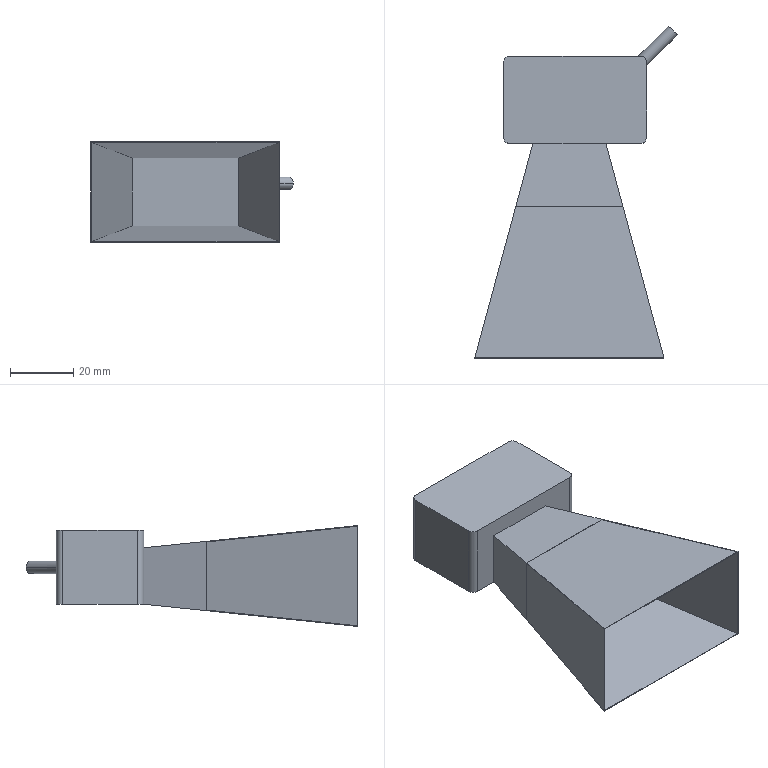Part | SolidWorks | features Blend 2, Extrusion 1, HoleWzd 1, ICE 1, Shell 1, Sweep 1 | 3 solids | 41 faces | box 64.206 x 105.323 x 32 mm | volume 42247 mm3 | plane 24 | cylinder 13 | cone 4 | commonest cylinder face diameters 4 x7 2.5 x4 7.5 x2
STEP:
#1=CARTESIAN_POINT('',(17.125,9.35,-3.25));
#2=VERTEX_POINT('',#1);
#3=CARTESIAN_POINT('',(14.625,9.35,-3.25));
#4=VERTEX_POINT('',#3);
#5=CARTESIAN_POINT('',(15.875,9.35,-3.25));
#6=DIRECTION('',(0.,0.,-1.));
#7=DIRECTION('',(-1.,0.,0.));
#8=AXIS2_PLACEMENT_3D('',#5,#6,#7);
#9=CIRCLE('',#8,1.25);
#10=EDGE_CURVE('',#2,#4,#9,.T.);
#11=ORIENTED_EDGE('',*,*,#10,.F.);
#12=CARTESIAN_POINT('',(17.125,9.35,-11.75));
#13=VERTEX_POINT('',#12);
#14=CARTESIAN_POINT('',(17.125,9.35,-11.75));
#15=DIRECTION('',(0.,0.,-1.));
#16=VECTOR('',#15,1000.);
#17=LINE('',#14,#16);
#18=EDGE_CURVE('',#2,#13,#17,.T.);
#19=ORIENTED_EDGE('',*,*,#18,.T.);
#20=CARTESIAN_POINT('',(14.625,9.35,-11.75));
#21=VERTEX_POINT('',#20);
#22=CARTESIAN_POINT('',(15.875,9.35,-11.75));
#23=DIRECTION('',(0.,0.,-1.));
#24=DIRECTION('',(-1.,0.,0.));
#25=AXIS2_PLACEMENT_3D('',#22,#23,#24);
#26=CIRCLE('',#25,1.25);
#27=EDGE_CURVE('',#13,#21,#26,.T.);
#28=ORIENTED_EDGE('',*,*,#27,.T.);
#29=CARTESIAN_POINT('',(14.625,9.35,-11.75));
#30=DIRECTION('',(0.,0.,-1.));
#31=VECTOR('',#30,1000.);
#32=LINE('',#29,#31);
#33=EDGE_CURVE('',#4,#21,#32,.T.);
#34=ORIENTED_EDGE('',*,*,#33,.F.);
#35=EDGE_LOOP('',(#11,#19,#28,#34));
#36=FACE_OUTER_BOUND('',#35,.T.);
#37=CARTESIAN_POINT('',(15.875,9.35,-11.75));
#38=DIRECTION('',(0.,0.,-1.));
#39=DIRECTION('',(-1.,0.,0.));
#40=AXIS2_PLACEMENT_3D('',#37,#38,#39);
#41=CYLINDRICAL_SURFACE('',#40,1.25);
#42=ADVANCED_FACE('',(#36),#41,.F.);
#43=CARTESIAN_POINT('',(15.875,9.35,-2.499));
#44=VERTEX_POINT('',#43);
#45=CARTESIAN_POINT('',(14.625,9.35,-3.25));
#46=DIRECTION('',(-0.8572,0.,-0.515));
#47=VECTOR('',#46,1000.);
#48=LINE('',#45,#47);
#49=EDGE_CURVE('',#44,#4,#48,.T.);
#50=ORIENTED_EDGE('',*,*,#49,.F.);
#51=CARTESIAN_POINT('',(17.125,9.35,-3.25));
#52=DIRECTION('',(0.8572,0.,-0.515));
#53=VECTOR('',#52,1000.);
#54=LINE('',#51,#53);
#55=EDGE_CURVE('',#44,#2,#54,.T.);
#56=ORIENTED_EDGE('',*,*,#55,.T.);
#57=ORIENTED_EDGE('',*,*,#10,.T.);
#58=EDGE_LOOP('',(#50,#56,#57));
#59=FACE_OUTER_BOUND('',#58,.T.);
#60=CARTESIAN_POINT('',(15.875,9.35,-3.25));
#61=DIRECTION('',(0.,0.,-1.));
#62=DIRECTION('',(-1.,0.,0.));
#63=AXIS2_PLACEMENT_3D('',#60,#61,#62);
#64=CONICAL_SURFACE('',#63,1.25,1.03);
#65=ADVANCED_FACE('',(#59),#64,.F.);
#66=CARTESIAN_POINT('',(-14.625,9.35,-3.25));
#67=VERTEX_POINT('',#66);
#68=CARTESIAN_POINT('',(-17.125,9.35,-3.25));
#69=VERTEX_POINT('',#68);
#70=CARTESIAN_POINT('',(-15.875,9.35,-3.25));
#71=DIRECTION('',(0.,0.,-1.));
#72=DIRECTION('',(-1.,0.,0.));
#73=AXIS2_PLACEMENT_3D('',#70,#71,#72);
#74=CIRCLE('',#73,1.25);
#75=EDGE_CURVE('',#67,#69,#74,.T.);
#76=ORIENTED_EDGE('',*,*,#75,.F.);
#77=CARTESIAN_POINT('',(-14.625,9.35,-11.75));
#78=VERTEX_POINT('',#77);
#79=CARTESIAN_POINT('',(-14.625,9.35,-11.75));
#80=DIRECTION('',(0.,0.,-1.));
#81=VECTOR('',#80,1000.);
#82=LINE('',#79,#81);
#83=EDGE_CURVE('',#67,#78,#82,.T.);
#84=ORIENTED_EDGE('',*,*,#83,.T.);
#85=CARTESIAN_POINT('',(-17.125,9.35,-11.75));
#86=VERTEX_POINT('',#85);
#87=CARTESIAN_POINT('',(-15.875,9.35,-11.75));
#88=DIRECTION('',(0.,0.,-1.));
#89=DIRECTION('',(-1.,0.,0.));
#90=AXIS2_PLACEMENT_3D('',#87,#88,#89);
#91=CIRCLE('',#90,1.25);
#92=EDGE_CURVE('',#78,#86,#91,.T.);
#93=ORIENTED_EDGE('',*,*,#92,.T.);
#94=CARTESIAN_POINT('',(-17.125,9.35,-11.75));
#95=DIRECTION('',(0.,0.,-1.));
#96=VECTOR('',#95,1000.);
#97=LINE('',#94,#96);
#98=EDGE_CURVE('',#69,#86,#97,.T.);
#99=ORIENTED_EDGE('',*,*,#98,.F.);
#100=EDGE_LOOP('',(#76,#84,#93,#99));
#101=FACE_OUTER_BOUND('',#100,.T.);
#102=CARTESIAN_POINT('',(-15.875,9.35,-11.75));
#103=DIRECTION('',(0.,0.,-1.));
#104=DIRECTION('',(-1.,0.,0.));
#105=AXIS2_PLACEMENT_3D('',#102,#103,#104);
#106=CYLINDRICAL_SURFACE('',#105,1.25);
#107=ADVANCED_FACE('',(#101),#106,.F.);
#108=CARTESIAN_POINT('',(-15.875,9.35,-2.499));
#109=VERTEX_POINT('',#108);
#110=CARTESIAN_POINT('',(-17.125,9.35,-3.25));
#111=DIRECTION('',(-0.8572,0.,-0.515));
#112=VECTOR('',#111,1000.);
#113=LINE('',#110,#112);
#114=EDGE_CURVE('',#109,#69,#113,.T.);
#115=ORIENTED_EDGE('',*,*,#114,.F.);
#116=CARTESIAN_POINT('',(-14.625,9.35,-3.25));
#117=DIRECTION('',(0.8572,0.,-0.515));
#118=VECTOR('',#117,1000.);
#119=LINE('',#116,#118);
#120=EDGE_CURVE('',#109,#67,#119,.T.);
#121=ORIENTED_EDGE('',*,*,#120,.T.);
#122=ORIENTED_EDGE('',*,*,#75,.T.);
#123=EDGE_LOOP('',(#115,#121,#122));
#124=FACE_OUTER_BOUND('',#123,.T.);
#125=CARTESIAN_POINT('',(-15.875,9.35,-3.25));
#126=DIRECTION('',(0.,0.,-1.));
#127=DIRECTION('',(-1.,0.,0.));
#128=AXIS2_PLACEMENT_3D('',#125,#126,#127);
#129=CONICAL_SURFACE('',#128,1.25,1.03);
#130=ADVANCED_FACE('',(#124),#129,.F.);
#131=CARTESIAN_POINT('',(-1.8,-8.85,1.));
#132=VERTEX_POINT('',#131);
#133=CARTESIAN_POINT('',(-1.8,-8.85,-6.5));
#134=VERTEX_POINT('',#133);
#135=CARTESIAN_POINT('',(-1.8,-8.85,-2.75));
#136=DIRECTION('',(0.,-1.,0.));
#137=DIRECTION('',(0.,0.,-1.));
#138=AXIS2_PLACEMENT_3D('',#135,#136,#137);
#139=CIRCLE('',#138,3.75);
#140=EDGE_CURVE('',#132,#134,#139,.T.);
#141=ORIENTED_EDGE('',*,*,#140,.F.);
#142=CARTESIAN_POINT('',(-1.8,-13.85,1.));
#143=VERTEX_POINT('',#142);
#144=CARTESIAN_POINT('',(-1.8,-8.85,1.));
#145=DIRECTION('',(0.,-1.,0.));
#146=VECTOR('',#145,1000.);
#147=LINE('',#144,#146);
#148=EDGE_CURVE('',#132,#143,#147,.T.);
#149=ORIENTED_EDGE('',*,*,#148,.T.);
#150=CARTESIAN_POINT('',(-1.8,-13.85,-6.5));
#151=VERTEX_POINT('',#150);
#152=CARTESIAN_POINT('',(-1.8,-13.85,-2.75));
#153=DIRECTION('',(0.,-1.,0.));
#154=DIRECTION('',(0.,0.,-1.));
#155=AXIS2_PLACEMENT_3D('',#152,#153,#154);
#156=CIRCLE('',#155,3.75);
#157=EDGE_CURVE('',#143,#151,#156,.T.);
#158=ORIENTED_EDGE('',*,*,#157,.T.);
#159=CARTESIAN_POINT('',(-1.8,-8.85,-6.5));
#160=DIRECTION('',(0.,-1.,0.));
#161=VECTOR('',#160,1000.);
#162=LINE('',#159,#161);
#163=EDGE_CURVE('',#134,#151,#162,.T.);
#164=ORIENTED_EDGE('',*,*,#163,.F.);
#165=EDGE_LOOP('',(#141,#149,#158,#164));
#166=FACE_OUTER_BOUND('',#165,.T.);
#167=CARTESIAN_POINT('',(-1.8,-8.85,-2.75));
#168=DIRECTION('',(0.,-1.,0.));
#169=DIRECTION('',(0.,0.,-1.));
#170=AXIS2_PLACEMENT_3D('',#167,#168,#169);
#171=CYLINDRICAL_SURFACE('',#170,3.75);
#172=ADVANCED_FACE('',(#166),#171,.F.);
#173=CARTESIAN_POINT('',(22.7,10.938,0.));
#174=VERTEX_POINT('',#173);
#175=CARTESIAN_POINT('',(22.7,11.85,1.471));
#176=VERTEX_POINT('',#175);
#177=CARTESIAN_POINT('',(22.7,10.938,0.));
#178=CARTESIAN_POINT('',(22.7,10.938,0.5672));
#179=CARTESIAN_POINT('',(22.7,11.26,1.087));
#180=CARTESIAN_POINT('',(22.7,11.85,1.471));
#181=(BOUNDED_CURVE()B_SPLINE_CURVE(3,(#177,#178,#179,#180),.UNSPECIFIED.,.F.,.F.)B_SPLINE_CURVE_WITH_KNOTS((4,4),(3.142,3.968),.UNSPECIFIED.)CURVE()GEOMETRIC_REPRESENTATION_ITEM()RATIONAL_B_SPLINE_CURVE((1.,0.9439,0.9439,1.))REPRESENTATION_ITEM(''));
#182=EDGE_CURVE('',#174,#176,#181,.T.);
#183=ORIENTED_EDGE('',*,*,#182,.F.);
#184=CARTESIAN_POINT('',(32.406,20.644,0.));
#185=VERTEX_POINT('',#184);
#186=CARTESIAN_POINT('',(21.8,10.038,0.));
#187=DIRECTION('',(0.7071,0.7071,0.));
#188=VECTOR('',#187,1000.);
#189=LINE('',#186,#188);
#190=EDGE_CURVE('',#174,#185,#189,.T.);
#191=ORIENTED_EDGE('',*,*,#190,.T.);
#192=CARTESIAN_POINT('',(29.578,23.473,0.));
#193=VERTEX_POINT('',#192);
#194=CARTESIAN_POINT('',(30.992,22.059,0.));
#195=DIRECTION('',(0.7071,0.7071,0.));
#196=DIRECTION('',(-0.7071,0.7071,0.));
#197=AXIS2_PLACEMENT_3D('',#194,#195,#196);
#198=CIRCLE('',#197,2.);
#199=EDGE_CURVE('',#193,#185,#198,.T.);
#200=ORIENTED_EDGE('',*,*,#199,.F.);
#201=CARTESIAN_POINT('',(19.955,13.85,0.));
#202=VERTEX_POINT('',#201);
#203=CARTESIAN_POINT('',(18.971,12.866,0.));
#204=DIRECTION('',(0.7071,0.7071,0.));
#205=VECTOR('',#204,1000.);
#206=LINE('',#203,#205);
#207=EDGE_CURVE('',#202,#193,#206,.T.);
#208=ORIENTED_EDGE('',*,*,#207,.F.);
#209=CARTESIAN_POINT('',(20.7,13.85,1.353));
#210=VERTEX_POINT('',#209);
#211=CARTESIAN_POINT('',(20.7,13.85,1.353));
#212=CARTESIAN_POINT('',(20.215,13.85,0.9792));
#213=CARTESIAN_POINT('',(19.955,13.85,0.5069));
#214=CARTESIAN_POINT('',(19.955,13.85,0.));
#215=(BOUNDED_CURVE()B_SPLINE_CURVE(3,(#211,#212,#213,#214),.UNSPECIFIED.,.F.,.F.)B_SPLINE_CURVE_WITH_KNOTS((4,4),(2.399,3.142),.UNSPECIFIED.)CURVE()GEOMETRIC_REPRESENTATION_ITEM()RATIONAL_B_SPLINE_CURVE((1.,0.9546,0.9546,1.))REPRESENTATION_ITEM(''));
#216=EDGE_CURVE('',#210,#202,#215,.T.);
#217=ORIENTED_EDGE('',*,*,#216,.F.);
#218=CARTESIAN_POINT('',(22.7,11.85,1.471));
#219=CARTESIAN_POINT('',(22.7,11.97,1.549));
#220=CARTESIAN_POINT('',(22.689,12.091,1.621));
#221=CARTESIAN_POINT('',(22.644,12.337,1.753));
#222=CARTESIAN_POINT('',(22.608,12.464,1.812));
#223=CARTESIAN_POINT('',(22.51,12.712,1.909));
#224=CARTESIAN_POINT('',(22.446,12.835,1.947));
#225=CARTESIAN_POINT('',(22.292,13.069,1.994));
#226=CARTESIAN_POINT('',(22.202,13.178,2.004));
#227=CARTESIAN_POINT('',(21.897,13.477,1.987));
#228=CARTESIAN_POINT('',(21.653,13.627,1.913));
#229=CARTESIAN_POINT('',(21.29,13.766,1.739));
#230=CARTESIAN_POINT('',(21.167,13.798,1.67));
#231=CARTESIAN_POINT('',(20.929,13.84,1.521));
#232=CARTESIAN_POINT('',(20.813,13.85,1.44));
#233=CARTESIAN_POINT('',(20.7,13.85,1.353));
#234=B_SPLINE_CURVE_WITH_KNOTS('',3,(#218,#219,#220,#221,#222,#223,#224,#225,#226,#227,#228,#229,#230,#231,#232,#233),.UNSPECIFIED.,.F.,.F.,(4,2,2,2,2,2,2,4),(0.,0.0004241,0.0008483,0.001272,0.001697,0.002545,0.002969,0.003393),.UNSPECIFIED.);
#235=EDGE_CURVE('',#176,#210,#234,.T.);
#236=ORIENTED_EDGE('',*,*,#235,.F.);
#237=EDGE_LOOP('',(#183,#191,#200,#208,#217,#236));
#238=FACE_OUTER_BOUND('',#237,.T.);
#239=CARTESIAN_POINT('',(20.385,11.452,0.));
#240=DIRECTION('',(0.7071,0.7071,0.));
#241=DIRECTION('',(-0.7071,0.7071,0.));
#242=AXIS2_PLACEMENT_3D('',#239,#240,#241);
#243=CYLINDRICAL_SURFACE('',#242,2.);
#244=ADVANCED_FACE('',(#238),#243,.T.);
#245=CARTESIAN_POINT('',(22.7,11.85,11.75));
#246=VERTEX_POINT('',#245);
#247=CARTESIAN_POINT('',(22.7,11.85,11.75));
#248=DIRECTION('',(0.,0.,-1.));
#249=VECTOR('',#248,1000.);
#250=LINE('',#247,#249);
#251=EDGE_CURVE('',#246,#176,#250,.T.);
#252=ORIENTED_EDGE('',*,*,#251,.T.);
#253=ORIENTED_EDGE('',*,*,#235,.T.);
#254=CARTESIAN_POINT('',(20.7,13.85,11.75));
#255=VERTEX_POINT('',#254);
#256=CARTESIAN_POINT('',(20.7,13.85,11.75));
#257=DIRECTION('',(0.,0.,-1.));
#258=VECTOR('',#257,1000.);
#259=LINE('',#256,#258);
#260=EDGE_CURVE('',#255,#210,#259,.T.);
#261=ORIENTED_EDGE('',*,*,#260,.F.);
#262=CARTESIAN_POINT('',(20.7,11.85,11.75));
#263=DIRECTION('',(0.,0.,1.));
#264=DIRECTION('',(1.,0.,0.));
#265=AXIS2_PLACEMENT_3D('',#262,#263,#264);
#266=CIRCLE('',#265,2.);
#267=EDGE_CURVE('',#246,#255,#266,.T.);
#268=ORIENTED_EDGE('',*,*,#267,.F.);
#269=EDGE_LOOP('',(#252,#253,#261,#268));
#270=FACE_OUTER_BOUND('',#269,.T.);
#271=CARTESIAN_POINT('',(20.7,11.85,11.75));
#272=DIRECTION('',(0.,0.,-1.));
#273=DIRECTION('',(-1.,0.,0.));
#274=AXIS2_PLACEMENT_3D('',#271,#272,#273);
#275=CYLINDRICAL_SURFACE('',#274,2.);
#276=ADVANCED_FACE('',(#270),#275,.T.);
#277=CARTESIAN_POINT('',(20.7,13.85,-1.353));
#278=VERTEX_POINT('',#277);
#279=CARTESIAN_POINT('',(20.7,13.85,-11.75));
#280=VERTEX_POINT('',#279);
#281=CARTESIAN_POINT('',(20.7,13.85,11.75));
#282=DIRECTION('',(0.,0.,-1.));
#283=VECTOR('',#282,1000.);
#284=LINE('',#281,#283);
#285=EDGE_CURVE('',#278,#280,#284,.T.);
#286=ORIENTED_EDGE('',*,*,#285,.F.);
#287=CARTESIAN_POINT('',(22.7,11.85,-1.471));
#288=VERTEX_POINT('',#287);
#289=CARTESIAN_POINT('',(20.7,13.85,-1.353));
#290=CARTESIAN_POINT('',(20.813,13.85,-1.44));
#291=CARTESIAN_POINT('',(20.929,13.84,-1.521));
#292=CARTESIAN_POINT('',(21.166,13.799,-1.67));
#293=CARTESIAN_POINT('',(21.288,13.766,-1.738));
#294=CARTESIAN_POINT('',(21.652,13.628,-1.912));
#295=CARTESIAN_POINT('',(21.894,13.479,-1.986));
#296=CARTESIAN_POINT('',(22.198,13.183,-2.004));
#297=CARTESIAN_POINT('',(22.29,13.071,-1.995));
#298=CARTESIAN_POINT('',(22.444,12.838,-1.948));
#299=CARTESIAN_POINT('',(22.509,12.714,-1.91));
#300=CARTESIAN_POINT('',(22.608,12.466,-1.813));
#301=CARTESIAN_POINT('',(22.643,12.339,-1.754));
#302=CARTESIAN_POINT('',(22.689,12.091,-1.622));
#303=CARTESIAN_POINT('',(22.7,11.97,-1.549));
#304=CARTESIAN_POINT('',(22.7,11.85,-1.471));
#305=B_SPLINE_CURVE_WITH_KNOTS('',3,(#289,#290,#291,#292,#293,#294,#295,#296,#297,#298,#299,#300,#301,#302,#303,#304),.UNSPECIFIED.,.F.,.F.,(4,2,2,2,2,2,2,4),(0.,0.0004239,0.0008479,0.001696,0.00212,0.002544,0.002968,0.003392),.UNSPECIFIED.);
#306=EDGE_CURVE('',#278,#288,#305,.T.);
#307=ORIENTED_EDGE('',*,*,#306,.T.);
#308=CARTESIAN_POINT('',(22.7,11.85,-11.75));
#309=VERTEX_POINT('',#308);
#310=CARTESIAN_POINT('',(22.7,11.85,11.75));
#311=DIRECTION('',(0.,0.,-1.));
#312=VECTOR('',#311,1000.);
#313=LINE('',#310,#312);
#314=EDGE_CURVE('',#288,#309,#313,.T.);
#315=ORIENTED_EDGE('',*,*,#314,.T.);
#316=CARTESIAN_POINT('',(20.7,11.85,-11.75));
#317=DIRECTION('',(0.,0.,1.));
#318=DIRECTION('',(1.,0.,0.));
#319=AXIS2_PLACEMENT_3D('',#316,#317,#318);
#320=CIRCLE('',#319,2.);
#321=EDGE_CURVE('',#309,#280,#320,.T.);
#322=ORIENTED_EDGE('',*,*,#321,.T.);
#323=EDGE_LOOP('',(#286,#307,#315,#322));
#324=FACE_OUTER_BOUND('',#323,.T.);
#325=CARTESIAN_POINT('',(20.7,11.85,11.75));
#326=DIRECTION('',(0.,0.,-1.));
#327=DIRECTION('',(-1.,0.,0.));
#328=AXIS2_PLACEMENT_3D('',#325,#326,#327);
#329=CYLINDRICAL_SURFACE('',#328,2.);
#330=ADVANCED_FACE('',(#324),#329,.T.);
#331=ORIENTED_EDGE('',*,*,#260,.T.);
#332=ORIENTED_EDGE('',*,*,#216,.T.);
#333=CARTESIAN_POINT('',(19.955,13.85,0.));
#334=CARTESIAN_POINT('',(19.955,13.85,-0.5069));
#335=CARTESIAN_POINT('',(20.215,13.85,-0.9792));
#336=CARTESIAN_POINT('',(20.7,13.85,-1.353));
#337=(BOUNDED_CURVE()B_SPLINE_CURVE(3,(#333,#334,#335,#336),.UNSPECIFIED.,.F.,.F.)B_SPLINE_CURVE_WITH_KNOTS((4,4),(3.142,3.884),.UNSPECIFIED.)CURVE()GEOMETRIC_REPRESENTATION_ITEM()RATIONAL_B_SPLINE_CURVE((1.,0.9546,0.9546,1.))REPRESENTATION_ITEM(''));
#338=EDGE_CURVE('',#202,#278,#337,.T.);
#339=ORIENTED_EDGE('',*,*,#338,.T.);
#340=ORIENTED_EDGE('',*,*,#285,.T.);
#341=CARTESIAN_POINT('',(-20.7,13.85,-11.75));
#342=VERTEX_POINT('',#341);
#343=CARTESIAN_POINT('',(-20.7,13.85,-11.75));
#344=DIRECTION('',(-1.,0.,0.));
#345=VECTOR('',#344,1000.);
#346=LINE('',#343,#345);
#347=EDGE_CURVE('',#280,#342,#346,.T.);
#348=ORIENTED_EDGE('',*,*,#347,.T.);
#349=CARTESIAN_POINT('',(-20.7,13.85,11.75));
#350=VERTEX_POINT('',#349);
#351=CARTESIAN_POINT('',(-20.7,13.85,11.75));
#352=DIRECTION('',(0.,0.,-1.));
#353=VECTOR('',#352,1000.);
#354=LINE('',#351,#353);
#355=EDGE_CURVE('',#350,#342,#354,.T.);
#356=ORIENTED_EDGE('',*,*,#355,.F.);
#357=CARTESIAN_POINT('',(-20.7,13.85,11.75));
#358=DIRECTION('',(-1.,0.,0.));
#359=VECTOR('',#358,1000.);
#360=LINE('',#357,#359);
#361=EDGE_CURVE('',#255,#350,#360,.T.);
#362=ORIENTED_EDGE('',*,*,#361,.F.);
#363=EDGE_LOOP('',(#331,#332,#339,#340,#348,#356,#362));
#364=FACE_OUTER_BOUND('',#363,.T.);
#365=CARTESIAN_POINT('',(-20.7,13.85,11.75));
#366=DIRECTION('',(0.,-1.,0.));
#367=DIRECTION('',(0.,0.,-1.));
#368=AXIS2_PLACEMENT_3D('',#365,#366,#367);
#369=PLANE('',#368);
#370=ADVANCED_FACE('',(#364),#369,.F.);
#371=CARTESIAN_POINT('',(-22.7,11.85,-11.75));
#372=VERTEX_POINT('',#371);
#373=CARTESIAN_POINT('',(-20.7,11.85,-11.75));
#374=DIRECTION('',(0.,0.,1.));
#375=DIRECTION('',(-1.,0.,0.));
#376=AXIS2_PLACEMENT_3D('',#373,#374,#375);
#377=CIRCLE('',#376,2.);
#378=EDGE_CURVE('',#342,#372,#377,.T.);
#379=ORIENTED_EDGE('',*,*,#378,.T.);
#380=CARTESIAN_POINT('',(-22.7,11.85,11.75));
#381=VERTEX_POINT('',#380);
#382=CARTESIAN_POINT('',(-22.7,11.85,11.75));
#383=DIRECTION('',(0.,0.,-1.));
#384=VECTOR('',#383,1000.);
#385=LINE('',#382,#384);
#386=EDGE_CURVE('',#381,#372,#385,.T.);
#387=ORIENTED_EDGE('',*,*,#386,.F.);
#388=CARTESIAN_POINT('',(-20.7,11.85,11.75));
#389=DIRECTION('',(0.,0.,1.));
#390=DIRECTION('',(-1.,0.,0.));
#391=AXIS2_PLACEMENT_3D('',#388,#389,#390);
#392=CIRCLE('',#391,2.);
#393=EDGE_CURVE('',#350,#381,#392,.T.);
#394=ORIENTED_EDGE('',*,*,#393,.F.);
#395=ORIENTED_EDGE('',*,*,#355,.T.);
#396=EDGE_LOOP('',(#379,#387,#394,#395));
#397=FACE_OUTER_BOUND('',#396,.T.);
#398=CARTESIAN_POINT('',(-20.7,11.85,11.75));
#399=DIRECTION('',(0.,0.,-1.));
#400=DIRECTION('',(-1.,0.,0.));
#401=AXIS2_PLACEMENT_3D('',#398,#399,#400);
#402=CYLINDRICAL_SURFACE('',#401,2.);
#403=ADVANCED_FACE('',(#397),#402,.T.);
#404=CARTESIAN_POINT('',(-22.7,-11.85,-11.75));
#405=VERTEX_POINT('',#404);
#406=CARTESIAN_POINT('',(-22.7,-11.85,-11.75));
#407=DIRECTION('',(0.,-1.,0.));
#408=VECTOR('',#407,1000.);
#409=LINE('',#406,#408);
#410=EDGE_CURVE('',#372,#405,#409,.T.);
#411=ORIENTED_EDGE('',*,*,#410,.T.);
#412=CARTESIAN_POINT('',(-22.7,-11.85,11.75));
#413=VERTEX_POINT('',#412);
#414=CARTESIAN_POINT('',(-22.7,-11.85,11.75));
#415=DIRECTION('',(0.,0.,-1.));
#416=VECTOR('',#415,1000.);
#417=LINE('',#414,#416);
#418=EDGE_CURVE('',#413,#405,#417,.T.);
#419=ORIENTED_EDGE('',*,*,#418,.F.);
#420=CARTESIAN_POINT('',(-22.7,-11.85,11.75));
#421=DIRECTION('',(0.,-1.,0.));
#422=VECTOR('',#421,1000.);
#423=LINE('',#420,#422);
#424=EDGE_CURVE('',#381,#413,#423,.T.);
#425=ORIENTED_EDGE('',*,*,#424,.F.);
#426=ORIENTED_EDGE('',*,*,#386,.T.);
#427=EDGE_LOOP('',(#411,#419,#425,#426));
#428=FACE_OUTER_BOUND('',#427,.T.);
#429=CARTESIAN_POINT('',(-22.7,-11.85,11.75));
#430=DIRECTION('',(1.,0.,0.));
#431=DIRECTION('',(0.,0.,-1.));
#432=AXIS2_PLACEMENT_3D('',#429,#430,#431);
#433=PLANE('',#432);
#434=ADVANCED_FACE('',(#428),#433,.F.);
#435=CARTESIAN_POINT('',(-20.7,-13.85,-11.75));
#436=VERTEX_POINT('',#435);
#437=CARTESIAN_POINT('',(-20.7,-11.85,-11.75));
#438=DIRECTION('',(0.,0.,1.));
#439=DIRECTION('',(1.,0.,0.));
#440=AXIS2_PLACEMENT_3D('',#437,#438,#439);
#441=CIRCLE('',#440,2.);
#442=EDGE_CURVE('',#405,#436,#441,.T.);
#443=ORIENTED_EDGE('',*,*,#442,.T.);
#444=CARTESIAN_POINT('',(-20.7,-13.85,11.75));
#445=VERTEX_POINT('',#444);
#446=CARTESIAN_POINT('',(-20.7,-13.85,11.75));
#447=DIRECTION('',(0.,0.,-1.));
#448=VECTOR('',#447,1000.);
#449=LINE('',#446,#448);
#450=EDGE_CURVE('',#445,#436,#449,.T.);
#451=ORIENTED_EDGE('',*,*,#450,.F.);
#452=CARTESIAN_POINT('',(-20.7,-11.85,11.75));
#453=DIRECTION('',(0.,0.,1.));
#454=DIRECTION('',(1.,0.,0.));
#455=AXIS2_PLACEMENT_3D('',#452,#453,#454);
#456=CIRCLE('',#455,2.);
#457=EDGE_CURVE('',#413,#445,#456,.T.);
#458=ORIENTED_EDGE('',*,*,#457,.F.);
#459=ORIENTED_EDGE('',*,*,#418,.T.);
#460=EDGE_LOOP('',(#443,#451,#458,#459));
#461=FACE_OUTER_BOUND('',#460,.T.);
#462=CARTESIAN_POINT('',(-20.7,-11.85,11.75));
#463=DIRECTION('',(0.,0.,-1.));
#464=DIRECTION('',(-1.,0.,0.));
#465=AXIS2_PLACEMENT_3D('',#462,#463,#464);
#466=CYLINDRICAL_SURFACE('',#465,2.);
#467=ADVANCED_FACE('',(#461),#466,.T.);
#468=CARTESIAN_POINT('',(-1.8,-13.85,-2.75));
#469=DIRECTION('',(0.,-1.,0.));
#470=DIRECTION('',(0.,0.,-1.));
#471=AXIS2_PLACEMENT_3D('',#468,#469,#470);
#472=CIRCLE('',#471,3.75);
#473=EDGE_CURVE('',#151,#143,#472,.T.);
#474=ORIENTED_EDGE('',*,*,#473,.F.);
#475=ORIENTED_EDGE('',*,*,#157,.F.);
#476=EDGE_LOOP('',(#474,#475));
#477=FACE_BOUND('',#476,.T.);
#478=CARTESIAN_POINT('',(20.7,-13.85,-11.75));
#479=VERTEX_POINT('',#478);
#480=CARTESIAN_POINT('',(-20.7,-13.85,-11.75));
#481=DIRECTION('',(1.,0.,0.));
#482=VECTOR('',#481,1000.);
#483=LINE('',#480,#482);
#484=EDGE_CURVE('',#436,#479,#483,.T.);
#485=ORIENTED_EDGE('',*,*,#484,.T.);
#486=CARTESIAN_POINT('',(20.7,-13.85,11.75));
#487=VERTEX_POINT('',#486);
#488=CARTESIAN_POINT('',(20.7,-13.85,11.75));
#489=DIRECTION('',(0.,0.,-1.));
#490=VECTOR('',#489,1000.);
#491=LINE('',#488,#490);
#492=EDGE_CURVE('',#487,#479,#491,.T.);
#493=ORIENTED_EDGE('',*,*,#492,.F.);
#494=CARTESIAN_POINT('',(-20.7,-13.85,11.75));
#495=DIRECTION('',(1.,0.,0.));
#496=VECTOR('',#495,1000.);
#497=LINE('',#494,#496);
#498=EDGE_CURVE('',#445,#487,#497,.T.);
#499=ORIENTED_EDGE('',*,*,#498,.F.);
#500=ORIENTED_EDGE('',*,*,#450,.T.);
#501=EDGE_LOOP('',(#485,#493,#499,#500));
#502=FACE_OUTER_BOUND('',#501,.T.);
#503=CARTESIAN_POINT('',(-20.7,-13.85,11.75));
#504=DIRECTION('',(0.,1.,0.));
#505=DIRECTION('',(0.,0.,1.));
#506=AXIS2_PLACEMENT_3D('',#503,#504,#505);
#507=PLANE('',#506);
#508=ADVANCED_FACE('',(#477,#502),#507,.F.);
#509=CARTESIAN_POINT('',(22.7,-11.85,-11.75));
#510=VERTEX_POINT('',#509);
#511=CARTESIAN_POINT('',(20.7,-11.85,-11.75));
#512=DIRECTION('',(0.,0.,1.));
#513=DIRECTION('',(1.,0.,0.));
#514=AXIS2_PLACEMENT_3D('',#511,#512,#513);
#515=CIRCLE('',#514,2.);
#516=EDGE_CURVE('',#479,#510,#515,.T.);
#517=ORIENTED_EDGE('',*,*,#516,.T.);
#518=CARTESIAN_POINT('',(22.7,-11.85,11.75));
#519=VERTEX_POINT('',#518);
#520=CARTESIAN_POINT('',(22.7,-11.85,11.75));
#521=DIRECTION('',(0.,0.,-1.));
#522=VECTOR('',#521,1000.);
#523=LINE('',#520,#522);
#524=EDGE_CURVE('',#519,#510,#523,.T.);
#525=ORIENTED_EDGE('',*,*,#524,.F.);
#526=CARTESIAN_POINT('',(20.7,-11.85,11.75));
#527=DIRECTION('',(0.,0.,1.));
#528=DIRECTION('',(1.,0.,0.));
#529=AXIS2_PLACEMENT_3D('',#526,#527,#528);
#530=CIRCLE('',#529,2.);
#531=EDGE_CURVE('',#487,#519,#530,.T.);
#532=ORIENTED_EDGE('',*,*,#531,.F.);
#533=ORIENTED_EDGE('',*,*,#492,.T.);
#534=EDGE_LOOP('',(#517,#525,#532,#533));
#535=FACE_OUTER_BOUND('',#534,.T.);
#536=CARTESIAN_POINT('',(20.7,-11.85,11.75));
#537=DIRECTION('',(0.,0.,-1.));
#538=DIRECTION('',(-1.,0.,0.));
#539=AXIS2_PLACEMENT_3D('',#536,#537,#538);
#540=CYLINDRICAL_SURFACE('',#539,2.);
#541=ADVANCED_FACE('',(#535),#540,.T.);
#542=ORIENTED_EDGE('',*,*,#314,.F.);
#543=CARTESIAN_POINT('',(22.7,11.85,-1.471));
#544=CARTESIAN_POINT('',(22.7,11.26,-1.087));
#545=CARTESIAN_POINT('',(22.7,10.938,-0.5672));
#546=CARTESIAN_POINT('',(22.7,10.938,0.));
#547=(BOUNDED_CURVE()B_SPLINE_CURVE(3,(#543,#544,#545,#546),.UNSPECIFIED.,.F.,.F.)B_SPLINE_CURVE_WITH_KNOTS((4,4),(2.315,3.142),.UNSPECIFIED.)CURVE()GEOMETRIC_REPRESENTATION_ITEM()RATIONAL_B_SPLINE_CURVE((1.,0.9439,0.9439,1.))REPRESENTATION_ITEM(''));
#548=EDGE_CURVE('',#288,#174,#547,.T.);
#549=ORIENTED_EDGE('',*,*,#548,.T.);
#550=ORIENTED_EDGE('',*,*,#182,.T.);
#551=ORIENTED_EDGE('',*,*,#251,.F.);
#552=CARTESIAN_POINT('',(22.7,-11.85,11.75));
#553=DIRECTION('',(0.,1.,0.));
#554=VECTOR('',#553,1000.);
#555=LINE('',#552,#554);
#556=EDGE_CURVE('',#519,#246,#555,.T.);
#557=ORIENTED_EDGE('',*,*,#556,.F.);
#558=ORIENTED_EDGE('',*,*,#524,.T.);
#559=CARTESIAN_POINT('',(22.7,-11.85,-11.75));
#560=DIRECTION('',(0.,1.,0.));
#561=VECTOR('',#560,1000.);
#562=LINE('',#559,#561);
#563=EDGE_CURVE('',#510,#309,#562,.T.);
#564=ORIENTED_EDGE('',*,*,#563,.T.);
#565=EDGE_LOOP('',(#542,#549,#550,#551,#557,#558,#564));
#566=FACE_OUTER_BOUND('',#565,.T.);
#567=CARTESIAN_POINT('',(22.7,-11.85,11.75));
#568=DIRECTION('',(-1.,0.,0.));
#569=DIRECTION('',(0.,0.,1.));
#570=AXIS2_PLACEMENT_3D('',#567,#568,#569);
#571=PLANE('',#570);
#572=ADVANCED_FACE('',(#566),#571,.F.);
#573=ORIENTED_EDGE('',*,*,#267,.T.);
#574=ORIENTED_EDGE('',*,*,#361,.T.);
#575=ORIENTED_EDGE('',*,*,#393,.T.);
#576=ORIENTED_EDGE('',*,*,#424,.T.);
#577=ORIENTED_EDGE('',*,*,#457,.T.);
#578=ORIENTED_EDGE('',*,*,#498,.T.);
#579=ORIENTED_EDGE('',*,*,#531,.T.);
#580=ORIENTED_EDGE('',*,*,#556,.T.);
#581=EDGE_LOOP('',(#573,#574,#575,#576,#577,#578,#579,#580));
#582=FACE_OUTER_BOUND('',#581,.T.);
#583=CARTESIAN_POINT('',(20.7,11.85,11.75));
#584=DIRECTION('',(0.,0.,1.));
#585=DIRECTION('',(1.,0.,0.));
#586=AXIS2_PLACEMENT_3D('',#583,#584,#585);
#587=PLANE('',#586);
#588=ADVANCED_FACE('',(#582),#587,.T.);
#589=CARTESIAN_POINT('',(15.875,9.35,-11.75));
#590=DIRECTION('',(0.,0.,-1.));
#591=DIRECTION('',(-1.,0.,0.));
#592=AXIS2_PLACEMENT_3D('',#589,#590,#591);
#593=CIRCLE('',#592,1.25);
#594=EDGE_CURVE('',#21,#13,#593,.T.);
#595=ORIENTED_EDGE('',*,*,#594,.F.);
#596=ORIENTED_EDGE('',*,*,#27,.F.);
#597=EDGE_LOOP('',(#595,#596));
#598=FACE_BOUND('',#597,.T.);
#599=CARTESIAN_POINT('',(-15.875,9.35,-11.75));
#600=DIRECTION('',(0.,0.,-1.));
#601=DIRECTION('',(-1.,0.,0.));
#602=AXIS2_PLACEMENT_3D('',#599,#600,#601);
#603=CIRCLE('',#602,1.25);
#604=EDGE_CURVE('',#86,#78,#603,.T.);
#605=ORIENTED_EDGE('',*,*,#604,.F.);
#606=ORIENTED_EDGE('',*,*,#92,.F.);
#607=EDGE_LOOP('',(#605,#606));
#608=FACE_BOUND('',#607,.T.);
#609=ORIENTED_EDGE('',*,*,#321,.F.);
#610=ORIENTED_EDGE('',*,*,#563,.F.);
#611=ORIENTED_EDGE('',*,*,#516,.F.);
#612=ORIENTED_EDGE('',*,*,#484,.F.);
#613=ORIENTED_EDGE('',*,*,#442,.F.);
#614=ORIENTED_EDGE('',*,*,#410,.F.);
#615=ORIENTED_EDGE('',*,*,#378,.F.);
#616=ORIENTED_EDGE('',*,*,#347,.F.);
#617=EDGE_LOOP('',(#609,#610,#611,#612,#613,#614,#615,#616));
#618=FACE_OUTER_BOUND('',#617,.T.);
#619=CARTESIAN_POINT('',(20.7,11.85,-11.75));
#620=DIRECTION('',(0.,0.,1.));
#621=DIRECTION('',(1.,0.,0.));
#622=AXIS2_PLACEMENT_3D('',#619,#620,#621);
#623=PLANE('',#622);
#624=ADVANCED_FACE('',(#598,#608,#618),#623,.F.);
#625=ORIENTED_EDGE('',*,*,#190,.F.);
#626=ORIENTED_EDGE('',*,*,#548,.F.);
#627=ORIENTED_EDGE('',*,*,#306,.F.);
#628=ORIENTED_EDGE('',*,*,#338,.F.);
#629=ORIENTED_EDGE('',*,*,#207,.T.);
#630=CARTESIAN_POINT('',(30.992,22.059,0.));
#631=DIRECTION('',(0.7071,0.7071,0.));
#632=DIRECTION('',(-0.7071,0.7071,0.));
#633=AXIS2_PLACEMENT_3D('',#630,#631,#632);
#634=CIRCLE('',#633,2.);
#635=EDGE_CURVE('',#185,#193,#634,.T.);
#636=ORIENTED_EDGE('',*,*,#635,.F.);
#637=EDGE_LOOP('',(#625,#626,#627,#628,#629,#636));
#638=FACE_OUTER_BOUND('',#637,.T.);
#639=CARTESIAN_POINT('',(20.385,11.452,0.));
#640=DIRECTION('',(0.7071,0.7071,0.));
#641=DIRECTION('',(-0.7071,0.7071,0.));
#642=AXIS2_PLACEMENT_3D('',#639,#640,#641);
#643=CYLINDRICAL_SURFACE('',#642,2.);
#644=ADVANCED_FACE('',(#638),#643,.T.);
#645=ORIENTED_EDGE('',*,*,#199,.T.);
#646=ORIENTED_EDGE('',*,*,#635,.T.);
#647=EDGE_LOOP('',(#645,#646));
#648=FACE_OUTER_BOUND('',#647,.T.);
#649=CARTESIAN_POINT('',(30.992,22.059,0.));
#650=DIRECTION('',(0.7071,0.7071,0.));
#651=DIRECTION('',(-0.7071,0.7071,0.));
#652=AXIS2_PLACEMENT_3D('',#649,#650,#651);
#653=PLANE('',#652);
#654=ADVANCED_FACE('',(#648),#653,.T.);
#655=ORIENTED_EDGE('',*,*,#148,.F.);
#656=CARTESIAN_POINT('',(-1.8,-8.85,-2.75));
#657=DIRECTION('',(0.,-1.,0.));
#658=DIRECTION('',(0.,0.,-1.));
#659=AXIS2_PLACEMENT_3D('',#656,#657,#658);
#660=CIRCLE('',#659,3.75);
#661=EDGE_CURVE('',#134,#132,#660,.T.);
#662=ORIENTED_EDGE('',*,*,#661,.F.);
#663=ORIENTED_EDGE('',*,*,#163,.T.);
#664=ORIENTED_EDGE('',*,*,#473,.T.);
#665=EDGE_LOOP('',(#655,#662,#663,#664));
#666=FACE_OUTER_BOUND('',#665,.T.);
#667=CARTESIAN_POINT('',(-1.8,-8.85,-2.75));
#668=DIRECTION('',(0.,-1.,0.));
#669=DIRECTION('',(0.,0.,-1.));
#670=AXIS2_PLACEMENT_3D('',#667,#668,#669);
#671=CYLINDRICAL_SURFACE('',#670,3.75);
#672=ADVANCED_FACE('',(#666),#671,.F.);
#673=ORIENTED_EDGE('',*,*,#661,.T.);
#674=ORIENTED_EDGE('',*,*,#140,.T.);
#675=EDGE_LOOP('',(#673,#674));
#676=FACE_OUTER_BOUND('',#675,.T.);
#677=CARTESIAN_POINT('',(-1.8,-8.85,-2.75));
#678=DIRECTION('',(0.,-1.,0.));
#679=DIRECTION('',(0.,0.,-1.));
#680=AXIS2_PLACEMENT_3D('',#677,#678,#679);
#681=PLANE('',#680);
#682=ADVANCED_FACE('',(#676),#681,.T.);
#683=ORIENTED_EDGE('',*,*,#120,.F.);
#684=ORIENTED_EDGE('',*,*,#114,.T.);
#685=CARTESIAN_POINT('',(-15.875,9.35,-3.25));
#686=DIRECTION('',(0.,0.,-1.));
#687=DIRECTION('',(-1.,0.,0.));
#688=AXIS2_PLACEMENT_3D('',#685,#686,#687);
#689=CIRCLE('',#688,1.25);
#690=EDGE_CURVE('',#69,#67,#689,.T.);
#691=ORIENTED_EDGE('',*,*,#690,.T.);
#692=EDGE_LOOP('',(#683,#684,#691));
#693=FACE_OUTER_BOUND('',#692,.T.);
#694=CARTESIAN_POINT('',(-15.875,9.35,-3.25));
#695=DIRECTION('',(0.,0.,-1.));
#696=DIRECTION('',(-1.,0.,0.));
#697=AXIS2_PLACEMENT_3D('',#694,#695,#696);
#698=CONICAL_SURFACE('',#697,1.25,1.03);
#699=ADVANCED_FACE('',(#693),#698,.F.);
#700=ORIENTED_EDGE('',*,*,#83,.F.);
#701=ORIENTED_EDGE('',*,*,#690,.F.);
#702=ORIENTED_EDGE('',*,*,#98,.T.);
#703=ORIENTED_EDGE('',*,*,#604,.T.);
#704=EDGE_LOOP('',(#700,#701,#702,#703));
#705=FACE_OUTER_BOUND('',#704,.T.);
#706=CARTESIAN_POINT('',(-15.875,9.35,-11.75));
#707=DIRECTION('',(0.,0.,-1.));
#708=DIRECTION('',(-1.,0.,0.));
#709=AXIS2_PLACEMENT_3D('',#706,#707,#708);
#710=CYLINDRICAL_SURFACE('',#709,1.25);
#711=ADVANCED_FACE('',(#705),#710,.F.);
#712=ORIENTED_EDGE('',*,*,#55,.F.);
#713=ORIENTED_EDGE('',*,*,#49,.T.);
#714=CARTESIAN_POINT('',(15.875,9.35,-3.25));
#715=DIRECTION('',(0.,0.,-1.));
#716=DIRECTION('',(-1.,0.,0.));
#717=AXIS2_PLACEMENT_3D('',#714,#715,#716);
#718=CIRCLE('',#717,1.25);
#719=EDGE_CURVE('',#4,#2,#718,.T.);
#720=ORIENTED_EDGE('',*,*,#719,.T.);
#721=EDGE_LOOP('',(#712,#713,#720));
#722=FACE_OUTER_BOUND('',#721,.T.);
#723=CARTESIAN_POINT('',(15.875,9.35,-3.25));
#724=DIRECTION('',(0.,0.,-1.));
#725=DIRECTION('',(-1.,0.,0.));
#726=AXIS2_PLACEMENT_3D('',#723,#724,#725);
#727=CONICAL_SURFACE('',#726,1.25,1.03);
#728=ADVANCED_FACE('',(#722),#727,.F.);
#729=ORIENTED_EDGE('',*,*,#18,.F.);
#730=ORIENTED_EDGE('',*,*,#719,.F.);
#731=ORIENTED_EDGE('',*,*,#33,.T.);
#732=ORIENTED_EDGE('',*,*,#594,.T.);
#733=EDGE_LOOP('',(#729,#730,#731,#732));
#734=FACE_OUTER_BOUND('',#733,.T.);
#735=CARTESIAN_POINT('',(15.875,9.35,-11.75));
#736=DIRECTION('',(0.,0.,-1.));
#737=DIRECTION('',(-1.,0.,0.));
#738=AXIS2_PLACEMENT_3D('',#735,#736,#737);
#739=CYLINDRICAL_SURFACE('',#738,1.25);
#740=ADVANCED_FACE('',(#734),#739,.F.);
#741=CLOSED_SHELL('',(#42,#65,#107,#130,#172,#244,#276,#330,#370,#403,#434,#467,#508,#541,#572,#588,#624,#644,#654,#672,#682,#699,#711,#728,#740));
#742=MANIFOLD_SOLID_BREP('',#741);
#743=CARTESIAN_POINT('',(-31.8,-81.85,13.25));
#744=VERTEX_POINT('',#743);
#745=CARTESIAN_POINT('',(-31.8,-81.85,-18.75));
#746=VERTEX_POINT('',#745);
#747=CARTESIAN_POINT('',(-31.8,-81.85,13.25));
#748=DIRECTION('',(0.,0.,-1.));
#749=VECTOR('',#748,1000.);
#750=LINE('',#747,#749);
#751=EDGE_CURVE('',#744,#746,#750,.T.);
#752=ORIENTED_EDGE('',*,*,#751,.T.);
#753=CARTESIAN_POINT('',(28.2,-81.85,-18.75));
#754=VERTEX_POINT('',#753);
#755=CARTESIAN_POINT('',(28.2,-81.85,-18.75));
#756=DIRECTION('',(1.,0.,0.));
#757=VECTOR('',#756,1000.);
#758=LINE('',#755,#757);
#759=EDGE_CURVE('',#746,#754,#758,.T.);
#760=ORIENTED_EDGE('',*,*,#759,.T.);
#761=CARTESIAN_POINT('',(28.2,-81.85,13.25));
#762=VERTEX_POINT('',#761);
#763=CARTESIAN_POINT('',(28.2,-81.85,13.25));
#764=DIRECTION('',(0.,0.,1.));
#765=VECTOR('',#764,1000.);
#766=LINE('',#763,#765);
#767=EDGE_CURVE('',#754,#762,#766,.T.);
#768=ORIENTED_EDGE('',*,*,#767,.T.);
#769=CARTESIAN_POINT('',(28.2,-81.85,13.25));
#770=DIRECTION('',(-1.,0.,0.));
#771=VECTOR('',#770,1000.);
#772=LINE('',#769,#771);
#773=EDGE_CURVE('',#762,#744,#772,.T.);
#774=ORIENTED_EDGE('',*,*,#773,.T.);
#775=EDGE_LOOP('',(#752,#760,#768,#774));
#776=FACE_OUTER_BOUND('',#775,.T.);
#777=CARTESIAN_POINT('',(-31.593,-81.85,13.049));
#778=VERTEX_POINT('',#777);
#779=CARTESIAN_POINT('',(-31.593,-81.85,-18.549));
#780=VERTEX_POINT('',#779);
#781=CARTESIAN_POINT('',(-31.593,-81.85,0.));
#782=DIRECTION('',(0.,0.,-1.));
#783=VECTOR('',#782,1000.);
#784=LINE('',#781,#783);
#785=EDGE_CURVE('',#778,#780,#784,.T.);
#786=ORIENTED_EDGE('',*,*,#785,.F.);
#787=CARTESIAN_POINT('',(27.993,-81.85,13.049));
#788=VERTEX_POINT('',#787);
#789=CARTESIAN_POINT('',(0.,-81.85,13.049));
#790=DIRECTION('',(-1.,0.,0.));
#791=VECTOR('',#790,1000.);
#792=LINE('',#789,#791);
#793=EDGE_CURVE('',#788,#778,#792,.T.);
#794=ORIENTED_EDGE('',*,*,#793,.F.);
#795=CARTESIAN_POINT('',(27.993,-81.85,-18.549));
#796=VERTEX_POINT('',#795);
#797=CARTESIAN_POINT('',(27.993,-81.85,0.));
#798=DIRECTION('',(0.,0.,1.));
#799=VECTOR('',#798,1000.);
#800=LINE('',#797,#799);
#801=EDGE_CURVE('',#796,#788,#800,.T.);
#802=ORIENTED_EDGE('',*,*,#801,.F.);
#803=CARTESIAN_POINT('',(0.,-81.85,-18.549));
#804=DIRECTION('',(1.,0.,0.));
#805=VECTOR('',#804,1000.);
#806=LINE('',#803,#805);
#807=EDGE_CURVE('',#780,#796,#806,.T.);
#808=ORIENTED_EDGE('',*,*,#807,.F.);
#809=EDGE_LOOP('',(#786,#794,#802,#808));
#810=FACE_BOUND('',#809,.T.);
#811=CARTESIAN_POINT('',(0.,-81.85,0.));
#812=DIRECTION('',(0.,1.,0.));
#813=DIRECTION('',(0.,0.,1.));
#814=AXIS2_PLACEMENT_3D('',#811,#812,#813);
#815=PLANE('',#814);
#816=ADVANCED_FACE('',(#776,#810),#815,.F.);
#817=CARTESIAN_POINT('',(-18.8,-33.85,8.25));
#818=VERTEX_POINT('',#817);
#819=CARTESIAN_POINT('',(-18.8,-33.85,-13.75));
#820=VERTEX_POINT('',#819);
#821=CARTESIAN_POINT('',(-18.8,-33.85,8.25));
#822=DIRECTION('',(0.,0.,-1.));
#823=VECTOR('',#822,1000.);
#824=LINE('',#821,#823);
#825=EDGE_CURVE('',#818,#820,#824,.T.);
#826=ORIENTED_EDGE('',*,*,#825,.F.);
#827=CARTESIAN_POINT('',(15.2,-33.85,8.25));
#828=VERTEX_POINT('',#827);
#829=CARTESIAN_POINT('',(15.2,-33.85,8.25));
#830=DIRECTION('',(-1.,0.,0.));
#831=VECTOR('',#830,1000.);
#832=LINE('',#829,#831);
#833=EDGE_CURVE('',#828,#818,#832,.T.);
#834=ORIENTED_EDGE('',*,*,#833,.F.);
#835=CARTESIAN_POINT('',(15.2,-33.85,-13.75));
#836=VERTEX_POINT('',#835);
#837=CARTESIAN_POINT('',(15.2,-33.85,8.25));
#838=DIRECTION('',(0.,0.,1.));
#839=VECTOR('',#838,1000.);
#840=LINE('',#837,#839);
#841=EDGE_CURVE('',#836,#828,#840,.T.);
#842=ORIENTED_EDGE('',*,*,#841,.F.);
#843=CARTESIAN_POINT('',(15.2,-33.85,-13.75));
#844=DIRECTION('',(1.,0.,0.));
#845=VECTOR('',#844,1000.);
#846=LINE('',#843,#845);
#847=EDGE_CURVE('',#820,#836,#846,.T.);
#848=ORIENTED_EDGE('',*,*,#847,.F.);
#849=EDGE_LOOP('',(#826,#834,#842,#848));
#850=FACE_OUTER_BOUND('',#849,.T.);
#851=CARTESIAN_POINT('',(14.993,-33.85,8.049));
#852=VERTEX_POINT('',#851);
#853=CARTESIAN_POINT('',(-18.593,-33.85,8.049));
#854=VERTEX_POINT('',#853);
#855=CARTESIAN_POINT('',(0.,-33.85,8.049));
#856=DIRECTION('',(-1.,0.,0.));
#857=VECTOR('',#856,1000.);
#858=LINE('',#855,#857);
#859=EDGE_CURVE('',#852,#854,#858,.T.);
#860=ORIENTED_EDGE('',*,*,#859,.T.);
#861=CARTESIAN_POINT('',(-18.593,-33.85,-13.549));
#862=VERTEX_POINT('',#861);
#863=CARTESIAN_POINT('',(-18.593,-33.85,0.));
#864=DIRECTION('',(0.,0.,-1.));
#865=VECTOR('',#864,1000.);
#866=LINE('',#863,#865);
#867=EDGE_CURVE('',#854,#862,#866,.T.);
#868=ORIENTED_EDGE('',*,*,#867,.T.);
#869=CARTESIAN_POINT('',(14.993,-33.85,-13.549));
#870=VERTEX_POINT('',#869);
#871=CARTESIAN_POINT('',(0.,-33.85,-13.549));
#872=DIRECTION('',(1.,0.,0.));
#873=VECTOR('',#872,1000.);
#874=LINE('',#871,#873);
#875=EDGE_CURVE('',#862,#870,#874,.T.);
#876=ORIENTED_EDGE('',*,*,#875,.T.);
#877=CARTESIAN_POINT('',(14.993,-33.85,0.));
#878=DIRECTION('',(0.,0.,1.));
#879=VECTOR('',#878,1000.);
#880=LINE('',#877,#879);
#881=EDGE_CURVE('',#870,#852,#880,.T.);
#882=ORIENTED_EDGE('',*,*,#881,.T.);
#883=EDGE_LOOP('',(#860,#868,#876,#882));
#884=FACE_BOUND('',#883,.T.);
#885=CARTESIAN_POINT('',(0.,-33.85,0.));
#886=DIRECTION('',(0.,1.,0.));
#887=DIRECTION('',(0.,0.,1.));
#888=AXIS2_PLACEMENT_3D('',#885,#886,#887);
#889=PLANE('',#888);
#890=ADVANCED_FACE('',(#850,#884),#889,.T.);
#891=CARTESIAN_POINT('',(-18.8,-33.85,8.25));
#892=DIRECTION('',(-0.2601,-0.9604,0.1));
#893=VECTOR('',#892,1000.);
#894=LINE('',#891,#893);
#895=EDGE_CURVE('',#818,#744,#894,.T.);
#896=ORIENTED_EDGE('',*,*,#895,.T.);
#897=ORIENTED_EDGE('',*,*,#773,.F.);
#898=CARTESIAN_POINT('',(15.2,-33.85,8.25));
#899=DIRECTION('',(0.2601,-0.9604,0.1));
#900=VECTOR('',#899,1000.);
#901=LINE('',#898,#900);
#902=EDGE_CURVE('',#828,#762,#901,.T.);
#903=ORIENTED_EDGE('',*,*,#902,.F.);
#904=ORIENTED_EDGE('',*,*,#833,.T.);
#905=EDGE_LOOP('',(#896,#897,#903,#904));
#906=FACE_OUTER_BOUND('',#905,.T.);
#907=CARTESIAN_POINT('',(0.,0.4868,4.673));
#908=DIRECTION('',(0.,-0.1036,-0.9946));
#909=DIRECTION('',(0.,0.9946,-0.1036));
#910=AXIS2_PLACEMENT_3D('',#907,#908,#909);
#911=PLANE('',#910);
#912=ADVANCED_FACE('',(#906),#911,.F.);
#913=ORIENTED_EDGE('',*,*,#902,.T.);
#914=ORIENTED_EDGE('',*,*,#767,.F.);
#915=CARTESIAN_POINT('',(15.2,-33.85,-13.75));
#916=DIRECTION('',(0.2601,-0.9604,-0.1));
#917=VECTOR('',#916,1000.);
#918=LINE('',#915,#917);
#919=EDGE_CURVE('',#836,#754,#918,.T.);
#920=ORIENTED_EDGE('',*,*,#919,.F.);
#921=ORIENTED_EDGE('',*,*,#841,.T.);
#922=EDGE_LOOP('',(#913,#914,#920,#921));
#923=FACE_OUTER_BOUND('',#922,.T.);
#924=CARTESIAN_POINT('',(5.62,1.522,0.));
#925=DIRECTION('',(-0.9652,-0.2614,0.));
#926=DIRECTION('',(0.2614,-0.9652,0.));
#927=AXIS2_PLACEMENT_3D('',#924,#925,#926);
#928=PLANE('',#927);
#929=ADVANCED_FACE('',(#923),#928,.F.);
#930=CARTESIAN_POINT('',(-18.8,-33.85,-13.75));
#931=DIRECTION('',(-0.2601,-0.9604,-0.1));
#932=VECTOR('',#931,1000.);
#933=LINE('',#930,#932);
#934=EDGE_CURVE('',#820,#746,#933,.T.);
#935=ORIENTED_EDGE('',*,*,#934,.T.);
#936=ORIENTED_EDGE('',*,*,#751,.F.);
#937=ORIENTED_EDGE('',*,*,#895,.F.);
#938=ORIENTED_EDGE('',*,*,#825,.T.);
#939=EDGE_LOOP('',(#935,#936,#937,#938));
#940=FACE_OUTER_BOUND('',#939,.T.);
#941=CARTESIAN_POINT('',(-8.974,2.43,0.));
#942=DIRECTION('',(0.9652,-0.2614,0.));
#943=DIRECTION('',(0.2614,0.9652,0.));
#944=AXIS2_PLACEMENT_3D('',#941,#942,#943);
#945=PLANE('',#944);
#946=ADVANCED_FACE('',(#940),#945,.F.);
#947=ORIENTED_EDGE('',*,*,#919,.T.);
#948=ORIENTED_EDGE('',*,*,#759,.F.);
#949=ORIENTED_EDGE('',*,*,#934,.F.);
#950=ORIENTED_EDGE('',*,*,#847,.T.);
#951=EDGE_LOOP('',(#947,#948,#949,#950));
#952=FACE_OUTER_BOUND('',#951,.T.);
#953=CARTESIAN_POINT('',(0.,1.054,-10.114));
#954=DIRECTION('',(0.,-0.1036,0.9946));
#955=DIRECTION('',(0.,-0.9946,-0.1036));
#956=AXIS2_PLACEMENT_3D('',#953,#954,#955);
#957=PLANE('',#956);
#958=ADVANCED_FACE('',(#952),#957,.F.);
#959=CARTESIAN_POINT('',(-8.67,2.789,4.232));
#960=DIRECTION('',(-0.2601,-0.9604,0.1));
#961=VECTOR('',#960,1000.);
#962=LINE('',#959,#961);
#963=EDGE_CURVE('',#854,#778,#962,.T.);
#964=ORIENTED_EDGE('',*,*,#963,.F.);
#965=ORIENTED_EDGE('',*,*,#859,.F.);
#966=CARTESIAN_POINT('',(5.313,1.89,4.326));
#967=DIRECTION('',(0.2601,-0.9604,0.1));
#968=VECTOR('',#967,1000.);
#969=LINE('',#966,#968);
#970=EDGE_CURVE('',#852,#788,#969,.T.);
#971=ORIENTED_EDGE('',*,*,#970,.T.);
#972=ORIENTED_EDGE('',*,*,#793,.T.);
#973=EDGE_LOOP('',(#964,#965,#971,#972));
#974=FACE_OUTER_BOUND('',#973,.T.);
#975=CARTESIAN_POINT('',(0.,0.4661,4.474));
#976=DIRECTION('',(0.,-0.1036,-0.9946));
#977=DIRECTION('',(0.,0.9946,-0.1036));
#978=AXIS2_PLACEMENT_3D('',#975,#976,#977);
#979=PLANE('',#978);
#980=ADVANCED_FACE('',(#974),#979,.T.);
#981=ORIENTED_EDGE('',*,*,#970,.F.);
#982=ORIENTED_EDGE('',*,*,#881,.F.);
#983=CARTESIAN_POINT('',(5.17,2.418,-9.771));
#984=DIRECTION('',(0.2601,-0.9604,-0.1));
#985=VECTOR('',#984,1000.);
#986=LINE('',#983,#985);
#987=EDGE_CURVE('',#870,#796,#986,.T.);
#988=ORIENTED_EDGE('',*,*,#987,.T.);
#989=ORIENTED_EDGE('',*,*,#801,.T.);
#990=EDGE_LOOP('',(#981,#982,#988,#989));
#991=FACE_OUTER_BOUND('',#990,.T.);
#992=CARTESIAN_POINT('',(5.427,1.47,0.));
#993=DIRECTION('',(-0.9652,-0.2614,0.));
#994=DIRECTION('',(0.2614,-0.9652,0.));
#995=AXIS2_PLACEMENT_3D('',#992,#993,#994);
#996=PLANE('',#995);
#997=ADVANCED_FACE('',(#991),#996,.T.);
#998=CARTESIAN_POINT('',(-8.527,3.317,-9.677));
#999=DIRECTION('',(-0.2601,-0.9604,-0.1));
#1000=VECTOR('',#999,1000.);
#1001=LINE('',#998,#1000);
#1002=EDGE_CURVE('',#862,#780,#1001,.T.);
#1003=ORIENTED_EDGE('',*,*,#1002,.F.);
#1004=ORIENTED_EDGE('',*,*,#867,.F.);
#1005=ORIENTED_EDGE('',*,*,#963,.T.);
#1006=ORIENTED_EDGE('',*,*,#785,.T.);
#1007=EDGE_LOOP('',(#1003,#1004,#1005,#1006));
#1008=FACE_OUTER_BOUND('',#1007,.T.);
#1009=CARTESIAN_POINT('',(-8.781,2.378,0.));
#1010=DIRECTION('',(0.9652,-0.2614,0.));
#1011=DIRECTION('',(0.2614,0.9652,0.));
#1012=AXIS2_PLACEMENT_3D('',#1009,#1010,#1011);
#1013=PLANE('',#1012);
#1014=ADVANCED_FACE('',(#1008),#1013,.T.);
#1015=ORIENTED_EDGE('',*,*,#987,.F.);
#1016=ORIENTED_EDGE('',*,*,#875,.F.);
#1017=ORIENTED_EDGE('',*,*,#1002,.T.);
#1018=ORIENTED_EDGE('',*,*,#807,.T.);
#1019=EDGE_LOOP('',(#1015,#1016,#1017,#1018));
#1020=FACE_OUTER_BOUND('',#1019,.T.);
#1021=CARTESIAN_POINT('',(0.,1.033,-9.915));
#1022=DIRECTION('',(0.,-0.1036,0.9946));
#1023=DIRECTION('',(0.,-0.9946,-0.1036));
#1024=AXIS2_PLACEMENT_3D('',#1021,#1022,#1023);
#1025=PLANE('',#1024);
#1026=ADVANCED_FACE('',(#1020),#1025,.T.);
#1027=CLOSED_SHELL('',(#816,#890,#912,#929,#946,#958,#980,#997,#1014,#1026));
#1028=MANIFOLD_SOLID_BREP('',#1027);
#1029=CARTESIAN_POINT('',(9.785,-13.85,6.21));
#1030=VERTEX_POINT('',#1029);
#1031=CARTESIAN_POINT('',(9.785,-13.85,-11.71));
#1032=VERTEX_POINT('',#1031);
#1033=CARTESIAN_POINT('',(9.785,-13.85,6.21));
#1034=DIRECTION('',(0.,0.,-1.));
#1035=VECTOR('',#1034,1000.);
#1036=LINE('',#1033,#1035);
#1037=EDGE_CURVE('',#1030,#1032,#1036,.T.);
#1038=ORIENTED_EDGE('',*,*,#1037,.T.);
#1039=CARTESIAN_POINT('',(-13.385,-13.85,-11.71));
#1040=VERTEX_POINT('',#1039);
#1041=CARTESIAN_POINT('',(-13.385,-13.85,-11.71));
#1042=DIRECTION('',(-1.,0.,0.));
#1043=VECTOR('',#1042,1000.);
#1044=LINE('',#1041,#1043);
#1045=EDGE_CURVE('',#1032,#1040,#1044,.T.);
#1046=ORIENTED_EDGE('',*,*,#1045,.T.);
#1047=CARTESIAN_POINT('',(-13.385,-13.85,6.21));
#1048=VERTEX_POINT('',#1047);
#1049=CARTESIAN_POINT('',(-13.385,-13.85,6.21));
#1050=DIRECTION('',(0.,0.,1.));
#1051=VECTOR('',#1050,1000.);
#1052=LINE('',#1049,#1051);
#1053=EDGE_CURVE('',#1040,#1048,#1052,.T.);
#1054=ORIENTED_EDGE('',*,*,#1053,.T.);
#1055=CARTESIAN_POINT('',(-13.385,-13.85,6.21));
#1056=DIRECTION('',(1.,0.,0.));
#1057=VECTOR('',#1056,1000.);
#1058=LINE('',#1055,#1057);
#1059=EDGE_CURVE('',#1048,#1030,#1058,.T.);
#1060=ORIENTED_EDGE('',*,*,#1059,.T.);
#1061=EDGE_LOOP('',(#1038,#1046,#1054,#1060));
#1062=FACE_OUTER_BOUND('',#1061,.T.);
#1063=CARTESIAN_POINT('',(0.,-13.85,0.));
#1064=DIRECTION('',(0.,-1.,0.));
#1065=DIRECTION('',(0.,0.,-1.));
#1066=AXIS2_PLACEMENT_3D('',#1063,#1064,#1065);
#1067=PLANE('',#1066);
#1068=ADVANCED_FACE('',(#1062),#1067,.F.);
#1069=CARTESIAN_POINT('',(-18.8,-33.85,8.25));
#1070=VERTEX_POINT('',#1069);
#1071=CARTESIAN_POINT('',(-18.8,-33.85,-13.75));
#1072=VERTEX_POINT('',#1071);
#1073=CARTESIAN_POINT('',(-18.8,-33.85,8.25));
#1074=DIRECTION('',(0.,0.,-1.));
#1075=VECTOR('',#1074,1000.);
#1076=LINE('',#1073,#1075);
#1077=EDGE_CURVE('',#1070,#1072,#1076,.T.);
#1078=ORIENTED_EDGE('',*,*,#1077,.T.);
#1079=CARTESIAN_POINT('',(15.2,-33.85,-13.75));
#1080=VERTEX_POINT('',#1079);
#1081=CARTESIAN_POINT('',(15.2,-33.85,-13.75));
#1082=DIRECTION('',(1.,0.,0.));
#1083=VECTOR('',#1082,1000.);
#1084=LINE('',#1081,#1083);
#1085=EDGE_CURVE('',#1072,#1080,#1084,.T.);
#1086=ORIENTED_EDGE('',*,*,#1085,.T.);
#1087=CARTESIAN_POINT('',(15.2,-33.85,8.25));
#1088=VERTEX_POINT('',#1087);
#1089=CARTESIAN_POINT('',(15.2,-33.85,8.25));
#1090=DIRECTION('',(0.,0.,1.));
#1091=VECTOR('',#1090,1000.);
#1092=LINE('',#1089,#1091);
#1093=EDGE_CURVE('',#1080,#1088,#1092,.T.);
#1094=ORIENTED_EDGE('',*,*,#1093,.T.);
#1095=CARTESIAN_POINT('',(15.2,-33.85,8.25));
#1096=DIRECTION('',(-1.,0.,0.));
#1097=VECTOR('',#1096,1000.);
#1098=LINE('',#1095,#1097);
#1099=EDGE_CURVE('',#1088,#1070,#1098,.T.);
#1100=ORIENTED_EDGE('',*,*,#1099,.T.);
#1101=EDGE_LOOP('',(#1078,#1086,#1094,#1100));
#1102=FACE_OUTER_BOUND('',#1101,.T.);
#1103=CARTESIAN_POINT('',(0.,-33.85,0.));
#1104=DIRECTION('',(0.,1.,0.));
#1105=DIRECTION('',(0.,0.,1.));
#1106=AXIS2_PLACEMENT_3D('',#1103,#1104,#1105);
#1107=PLANE('',#1106);
#1108=ADVANCED_FACE('',(#1102),#1107,.F.);
#1109=CARTESIAN_POINT('',(-18.8,-33.85,8.25));
#1110=DIRECTION('',(0.2601,0.9606,-0.09798));
#1111=VECTOR('',#1110,1000.);
#1112=LINE('',#1109,#1111);
#1113=EDGE_CURVE('',#1070,#1048,#1112,.T.);
#1114=ORIENTED_EDGE('',*,*,#1113,.T.);
#1115=ORIENTED_EDGE('',*,*,#1053,.F.);
#1116=CARTESIAN_POINT('',(-18.8,-33.85,-13.75));
#1117=DIRECTION('',(0.2601,0.9606,0.09798));
#1118=VECTOR('',#1117,1000.);
#1119=LINE('',#1116,#1118);
#1120=EDGE_CURVE('',#1072,#1040,#1119,.T.);
#1121=ORIENTED_EDGE('',*,*,#1120,.F.);
#1122=ORIENTED_EDGE('',*,*,#1077,.F.);
#1123=EDGE_LOOP('',(#1114,#1115,#1121,#1122));
#1124=FACE_OUTER_BOUND('',#1123,.T.);
#1125=CARTESIAN_POINT('',(-8.977,2.431,0.));
#1126=DIRECTION('',(0.9652,-0.2613,0.));
#1127=DIRECTION('',(0.2613,0.9652,0.));
#1128=AXIS2_PLACEMENT_3D('',#1125,#1126,#1127);
#1129=PLANE('',#1128);
#1130=ADVANCED_FACE('',(#1124),#1129,.F.);
#1131=ORIENTED_EDGE('',*,*,#1120,.T.);
#1132=ORIENTED_EDGE('',*,*,#1045,.F.);
#1133=CARTESIAN_POINT('',(15.2,-33.85,-13.75));
#1134=DIRECTION('',(-0.2601,0.9606,0.09798));
#1135=VECTOR('',#1134,1000.);
#1136=LINE('',#1133,#1135);
#1137=EDGE_CURVE('',#1080,#1032,#1136,.T.);
#1138=ORIENTED_EDGE('',*,*,#1137,.F.);
#1139=ORIENTED_EDGE('',*,*,#1085,.F.);
#1140=EDGE_LOOP('',(#1131,#1132,#1138,#1139));
#1141=FACE_OUTER_BOUND('',#1140,.T.);
#1142=CARTESIAN_POINT('',(0.,1.04,-10.191));
#1143=DIRECTION('',(0.,-0.1015,0.9948));
#1144=DIRECTION('',(0.,-0.9948,-0.1015));
#1145=AXIS2_PLACEMENT_3D('',#1142,#1143,#1144);
#1146=PLANE('',#1145);
#1147=ADVANCED_FACE('',(#1141),#1146,.F.);
#1148=CARTESIAN_POINT('',(15.2,-33.85,8.25));
#1149=DIRECTION('',(-0.2601,0.9606,-0.09798));
#1150=VECTOR('',#1149,1000.);
#1151=LINE('',#1148,#1150);
#1152=EDGE_CURVE('',#1088,#1030,#1151,.T.);
#1153=ORIENTED_EDGE('',*,*,#1152,.T.);
#1154=ORIENTED_EDGE('',*,*,#1059,.F.);
#1155=ORIENTED_EDGE('',*,*,#1113,.F.);
#1156=ORIENTED_EDGE('',*,*,#1099,.F.);
#1157=EDGE_LOOP('',(#1153,#1154,#1155,#1156));
#1158=FACE_OUTER_BOUND('',#1157,.T.);
#1159=CARTESIAN_POINT('',(0.,0.4843,4.748));
#1160=DIRECTION('',(0.,-0.1015,-0.9948));
#1161=DIRECTION('',(0.,0.9948,-0.1015));
#1162=AXIS2_PLACEMENT_3D('',#1159,#1160,#1161);
#1163=PLANE('',#1162);
#1164=ADVANCED_FACE('',(#1158),#1163,.F.);
#1165=ORIENTED_EDGE('',*,*,#1137,.T.);
#1166=ORIENTED_EDGE('',*,*,#1037,.F.);
#1167=ORIENTED_EDGE('',*,*,#1152,.F.);
#1168=ORIENTED_EDGE('',*,*,#1093,.F.);
#1169=EDGE_LOOP('',(#1165,#1166,#1167,#1168));
#1170=FACE_OUTER_BOUND('',#1169,.T.);
#1171=CARTESIAN_POINT('',(5.623,1.522,0.));
#1172=DIRECTION('',(-0.9652,-0.2613,0.));
#1173=DIRECTION('',(0.2613,-0.9652,0.));
#1174=AXIS2_PLACEMENT_3D('',#1171,#1172,#1173);
#1175=PLANE('',#1174);
#1176=ADVANCED_FACE('',(#1170),#1175,.F.);
#1177=CLOSED_SHELL('',(#1068,#1108,#1130,#1147,#1164,#1176));
#1178=MANIFOLD_SOLID_BREP('',#1177);
#1179=CARTESIAN_POINT('',(0.,0.,0.));
#1180=DIRECTION('',(0.,0.,1.));
#1181=DIRECTION('',(1.,0.,0.));
#1182=AXIS2_PLACEMENT_3D('',#1179,#1180,#1181);
#1183=(LENGTH_UNIT()NAMED_UNIT(*)SI_UNIT(.MILLI.,.METRE.));
#1184=UNCERTAINTY_MEASURE_WITH_UNIT(LENGTH_MEASURE(0.00001),#1183,'','');
#1185=(NAMED_UNIT(*)PLANE_ANGLE_UNIT()SI_UNIT($,.RADIAN.));
#1186=(NAMED_UNIT(*)SI_UNIT($,.STERADIAN.)SOLID_ANGLE_UNIT());
#1187=(GEOMETRIC_REPRESENTATION_CONTEXT(3)GLOBAL_UNCERTAINTY_ASSIGNED_CONTEXT((#1184))GLOBAL_UNIT_ASSIGNED_CONTEXT((#1183,#1185,#1186))REPRESENTATION_CONTEXT('',''));
#1188=ADVANCED_BREP_SHAPE_REPRESENTATION('',(#742,#1028,#1178,#1182),#1187);